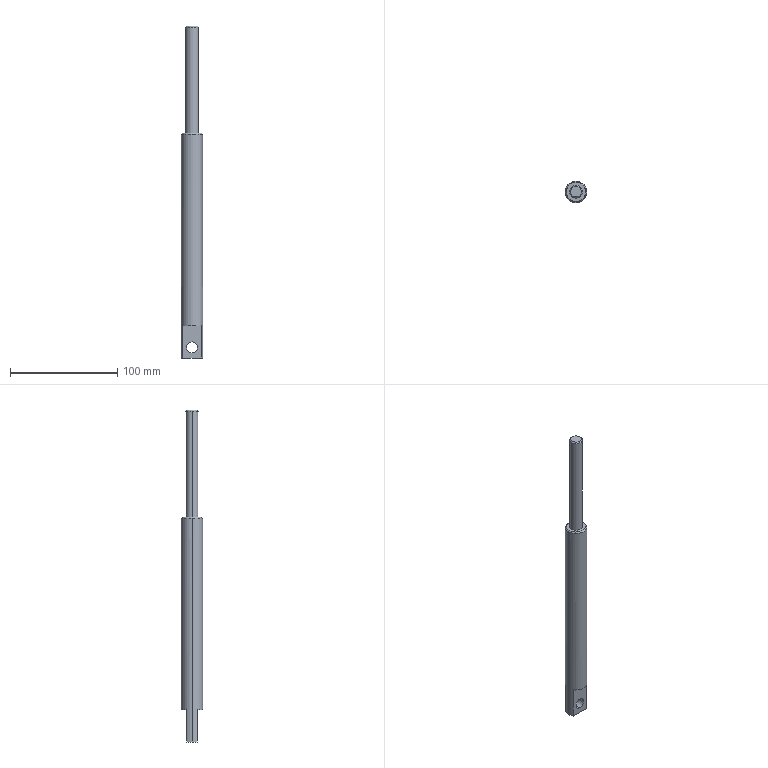Part | SolidWorks | features ICE 3, Chamfer 1, Extrusion 1 | 1 solid | 17 faces | box 20 x 20 x 310 mm | volume 72765 mm3 | plane 7 | cylinder 6 | cone 4 | commonest cylinder face diameters 10 x2 12 x2 20 x2
STEP:
#1=CARTESIAN_POINT('',(9.,0.,210.));
#2=VERTEX_POINT('',#1);
#3=CARTESIAN_POINT('',(-9.,0.,210.));
#4=VERTEX_POINT('',#3);
#5=CARTESIAN_POINT('',(0.,0.,210.));
#6=DIRECTION('',(0.,0.,1.));
#7=DIRECTION('',(1.,0.,0.));
#8=AXIS2_PLACEMENT_3D('',#5,#6,#7);
#9=CIRCLE('',#8,9.);
#10=EDGE_CURVE('',#2,#4,#9,.T.);
#11=ORIENTED_EDGE('',*,*,#10,.F.);
#12=CARTESIAN_POINT('',(10.,0.,209.));
#13=VERTEX_POINT('',#12);
#14=CARTESIAN_POINT('',(9.,0.,210.));
#15=DIRECTION('',(0.7071,0.,-0.7071));
#16=VECTOR('',#15,1000.);
#17=LINE('',#14,#16);
#18=EDGE_CURVE('',#2,#13,#17,.T.);
#19=ORIENTED_EDGE('',*,*,#18,.T.);
#20=CARTESIAN_POINT('',(-10.,0.,209.));
#21=VERTEX_POINT('',#20);
#22=CARTESIAN_POINT('',(0.,0.,209.));
#23=DIRECTION('',(0.,0.,-1.));
#24=DIRECTION('',(1.,0.,0.));
#25=AXIS2_PLACEMENT_3D('',#22,#23,#24);
#26=CIRCLE('',#25,10.);
#27=EDGE_CURVE('',#21,#13,#26,.T.);
#28=ORIENTED_EDGE('',*,*,#27,.F.);
#29=CARTESIAN_POINT('',(-9.,0.,210.));
#30=DIRECTION('',(-0.7071,0.,-0.7071));
#31=VECTOR('',#30,1000.);
#32=LINE('',#29,#31);
#33=EDGE_CURVE('',#4,#21,#32,.T.);
#34=ORIENTED_EDGE('',*,*,#33,.F.);
#35=EDGE_LOOP('',(#11,#19,#28,#34));
#36=FACE_OUTER_BOUND('',#35,.T.);
#37=CARTESIAN_POINT('',(0.,0.,210.));
#38=DIRECTION('',(0.,0.,-1.));
#39=DIRECTION('',(-1.,0.,0.));
#40=AXIS2_PLACEMENT_3D('',#37,#38,#39);
#41=CONICAL_SURFACE('',#40,9.,0.7854);
#42=ADVANCED_FACE('',(#36),#41,.T.);
#43=CARTESIAN_POINT('',(5.,0.,310.));
#44=VERTEX_POINT('',#43);
#45=CARTESIAN_POINT('',(-5.,0.,310.));
#46=VERTEX_POINT('',#45);
#47=CARTESIAN_POINT('',(0.,0.,310.));
#48=DIRECTION('',(0.,0.,1.));
#49=DIRECTION('',(1.,0.,0.));
#50=AXIS2_PLACEMENT_3D('',#47,#48,#49);
#51=CIRCLE('',#50,5.);
#52=EDGE_CURVE('',#44,#46,#51,.T.);
#53=ORIENTED_EDGE('',*,*,#52,.F.);
#54=CARTESIAN_POINT('',(6.,0.,309.));
#55=VERTEX_POINT('',#54);
#56=CARTESIAN_POINT('',(5.,0.,310.));
#57=DIRECTION('',(0.7071,0.,-0.7071));
#58=VECTOR('',#57,1000.);
#59=LINE('',#56,#58);
#60=EDGE_CURVE('',#44,#55,#59,.T.);
#61=ORIENTED_EDGE('',*,*,#60,.T.);
#62=CARTESIAN_POINT('',(-6.,0.,309.));
#63=VERTEX_POINT('',#62);
#64=CARTESIAN_POINT('',(0.,0.,309.));
#65=DIRECTION('',(0.,0.,-1.));
#66=DIRECTION('',(1.,0.,0.));
#67=AXIS2_PLACEMENT_3D('',#64,#65,#66);
#68=CIRCLE('',#67,6.);
#69=EDGE_CURVE('',#63,#55,#68,.T.);
#70=ORIENTED_EDGE('',*,*,#69,.F.);
#71=CARTESIAN_POINT('',(-5.,0.,310.));
#72=DIRECTION('',(-0.7071,0.,-0.7071));
#73=VECTOR('',#72,1000.);
#74=LINE('',#71,#73);
#75=EDGE_CURVE('',#46,#63,#74,.T.);
#76=ORIENTED_EDGE('',*,*,#75,.F.);
#77=EDGE_LOOP('',(#53,#61,#70,#76));
#78=FACE_OUTER_BOUND('',#77,.T.);
#79=CARTESIAN_POINT('',(0.,0.,310.));
#80=DIRECTION('',(0.,0.,-1.));
#81=DIRECTION('',(-1.,0.,0.));
#82=AXIS2_PLACEMENT_3D('',#79,#80,#81);
#83=CONICAL_SURFACE('',#82,5.,0.7854);
#84=ADVANCED_FACE('',(#78),#83,.T.);
#85=ORIENTED_EDGE('',*,*,#69,.T.);
#86=CARTESIAN_POINT('',(6.,0.,210.));
#87=VERTEX_POINT('',#86);
#88=CARTESIAN_POINT('',(6.,0.,310.));
#89=DIRECTION('',(0.,0.,-1.));
#90=VECTOR('',#89,1000.);
#91=LINE('',#88,#90);
#92=EDGE_CURVE('',#55,#87,#91,.T.);
#93=ORIENTED_EDGE('',*,*,#92,.T.);
#94=CARTESIAN_POINT('',(-6.,0.,210.));
#95=VERTEX_POINT('',#94);
#96=CARTESIAN_POINT('',(0.,0.,210.));
#97=DIRECTION('',(0.,0.,1.));
#98=DIRECTION('',(1.,0.,0.));
#99=AXIS2_PLACEMENT_3D('',#96,#97,#98);
#100=CIRCLE('',#99,6.);
#101=EDGE_CURVE('',#87,#95,#100,.T.);
#102=ORIENTED_EDGE('',*,*,#101,.T.);
#103=CARTESIAN_POINT('',(-6.,0.,310.));
#104=DIRECTION('',(0.,0.,-1.));
#105=VECTOR('',#104,1000.);
#106=LINE('',#103,#105);
#107=EDGE_CURVE('',#63,#95,#106,.T.);
#108=ORIENTED_EDGE('',*,*,#107,.F.);
#109=EDGE_LOOP('',(#85,#93,#102,#108));
#110=FACE_OUTER_BOUND('',#109,.T.);
#111=CARTESIAN_POINT('',(0.,0.,310.));
#112=DIRECTION('',(0.,0.,-1.));
#113=DIRECTION('',(-1.,0.,0.));
#114=AXIS2_PLACEMENT_3D('',#111,#112,#113);
#115=CYLINDRICAL_SURFACE('',#114,6.);
#116=ADVANCED_FACE('',(#110),#115,.T.);
#117=CARTESIAN_POINT('',(0.,-5.,5.));
#118=VERTEX_POINT('',#117);
#119=CARTESIAN_POINT('',(0.,-5.,15.));
#120=VERTEX_POINT('',#119);
#121=CARTESIAN_POINT('',(0.,-5.,10.));
#122=DIRECTION('',(0.,1.,0.));
#123=DIRECTION('',(0.,0.,-1.));
#124=AXIS2_PLACEMENT_3D('',#121,#122,#123);
#125=CIRCLE('',#124,5.);
#126=EDGE_CURVE('',#118,#120,#125,.T.);
#127=ORIENTED_EDGE('',*,*,#126,.F.);
#128=CARTESIAN_POINT('',(0.,5.,5.));
#129=VERTEX_POINT('',#128);
#130=CARTESIAN_POINT('',(0.,-10.,5.));
#131=DIRECTION('',(0.,1.,0.));
#132=VECTOR('',#131,1000.);
#133=LINE('',#130,#132);
#134=EDGE_CURVE('',#118,#129,#133,.T.);
#135=ORIENTED_EDGE('',*,*,#134,.T.);
#136=CARTESIAN_POINT('',(0.,5.,15.));
#137=VERTEX_POINT('',#136);
#138=CARTESIAN_POINT('',(0.,5.,10.));
#139=DIRECTION('',(0.,-1.,0.));
#140=DIRECTION('',(0.,0.,1.));
#141=AXIS2_PLACEMENT_3D('',#138,#139,#140);
#142=CIRCLE('',#141,5.);
#143=EDGE_CURVE('',#137,#129,#142,.T.);
#144=ORIENTED_EDGE('',*,*,#143,.F.);
#145=CARTESIAN_POINT('',(0.,-10.,15.));
#146=DIRECTION('',(0.,1.,0.));
#147=VECTOR('',#146,1000.);
#148=LINE('',#145,#147);
#149=EDGE_CURVE('',#120,#137,#148,.T.);
#150=ORIENTED_EDGE('',*,*,#149,.F.);
#151=EDGE_LOOP('',(#127,#135,#144,#150));
#152=FACE_OUTER_BOUND('',#151,.T.);
#153=CARTESIAN_POINT('',(0.,-10.,10.));
#154=DIRECTION('',(0.,1.,0.));
#155=DIRECTION('',(0.,0.,1.));
#156=AXIS2_PLACEMENT_3D('',#153,#154,#155);
#157=CYLINDRICAL_SURFACE('',#156,5.);
#158=ADVANCED_FACE('',(#152),#157,.F.);
#159=ORIENTED_EDGE('',*,*,#27,.T.);
#160=CARTESIAN_POINT('',(10.,0.,0.));
#161=VERTEX_POINT('',#160);
#162=CARTESIAN_POINT('',(10.,0.,210.));
#163=DIRECTION('',(0.,0.,-1.));
#164=VECTOR('',#163,1000.);
#165=LINE('',#162,#164);
#166=EDGE_CURVE('',#13,#161,#165,.T.);
#167=ORIENTED_EDGE('',*,*,#166,.T.);
#168=CARTESIAN_POINT('',(8.66,5.,0.));
#169=VERTEX_POINT('',#168);
#170=CARTESIAN_POINT('',(0.,0.,0.));
#171=DIRECTION('',(0.,0.,1.));
#172=DIRECTION('',(1.,0.,0.));
#173=AXIS2_PLACEMENT_3D('',#170,#171,#172);
#174=CIRCLE('',#173,10.);
#175=EDGE_CURVE('',#161,#169,#174,.T.);
#176=ORIENTED_EDGE('',*,*,#175,.T.);
#177=CARTESIAN_POINT('',(8.66,5.,30.));
#178=VERTEX_POINT('',#177);
#179=CARTESIAN_POINT('',(8.66,5.,210.));
#180=DIRECTION('',(0.,0.,-1.));
#181=VECTOR('',#180,1000.);
#182=LINE('',#179,#181);
#183=EDGE_CURVE('',#178,#169,#182,.T.);
#184=ORIENTED_EDGE('',*,*,#183,.F.);
#185=CARTESIAN_POINT('',(-8.66,5.,30.));
#186=VERTEX_POINT('',#185);
#187=CARTESIAN_POINT('',(0.,0.,30.));
#188=DIRECTION('',(0.,0.,-1.));
#189=DIRECTION('',(-1.,0.,0.));
#190=AXIS2_PLACEMENT_3D('',#187,#188,#189);
#191=CIRCLE('',#190,10.);
#192=EDGE_CURVE('',#186,#178,#191,.T.);
#193=ORIENTED_EDGE('',*,*,#192,.F.);
#194=CARTESIAN_POINT('',(-8.66,5.,0.));
#195=VERTEX_POINT('',#194);
#196=CARTESIAN_POINT('',(-8.66,5.,210.));
#197=DIRECTION('',(0.,0.,1.));
#198=VECTOR('',#197,1000.);
#199=LINE('',#196,#198);
#200=EDGE_CURVE('',#195,#186,#199,.T.);
#201=ORIENTED_EDGE('',*,*,#200,.F.);
#202=CARTESIAN_POINT('',(-10.,0.,0.));
#203=VERTEX_POINT('',#202);
#204=CARTESIAN_POINT('',(0.,0.,0.));
#205=DIRECTION('',(0.,0.,1.));
#206=DIRECTION('',(1.,0.,0.));
#207=AXIS2_PLACEMENT_3D('',#204,#205,#206);
#208=CIRCLE('',#207,10.);
#209=EDGE_CURVE('',#195,#203,#208,.T.);
#210=ORIENTED_EDGE('',*,*,#209,.T.);
#211=CARTESIAN_POINT('',(-10.,0.,210.));
#212=DIRECTION('',(0.,0.,-1.));
#213=VECTOR('',#212,1000.);
#214=LINE('',#211,#213);
#215=EDGE_CURVE('',#21,#203,#214,.T.);
#216=ORIENTED_EDGE('',*,*,#215,.F.);
#217=EDGE_LOOP('',(#159,#167,#176,#184,#193,#201,#210,#216));
#218=FACE_OUTER_BOUND('',#217,.T.);
#219=CARTESIAN_POINT('',(0.,0.,210.));
#220=DIRECTION('',(0.,0.,-1.));
#221=DIRECTION('',(-1.,0.,0.));
#222=AXIS2_PLACEMENT_3D('',#219,#220,#221);
#223=CYLINDRICAL_SURFACE('',#222,10.);
#224=ADVANCED_FACE('',(#218),#223,.T.);
#225=ORIENTED_EDGE('',*,*,#166,.F.);
#226=CARTESIAN_POINT('',(0.,0.,209.));
#227=DIRECTION('',(0.,0.,-1.));
#228=DIRECTION('',(1.,0.,0.));
#229=AXIS2_PLACEMENT_3D('',#226,#227,#228);
#230=CIRCLE('',#229,10.);
#231=EDGE_CURVE('',#13,#21,#230,.T.);
#232=ORIENTED_EDGE('',*,*,#231,.T.);
#233=ORIENTED_EDGE('',*,*,#215,.T.);
#234=CARTESIAN_POINT('',(-8.66,-5.,0.));
#235=VERTEX_POINT('',#234);
#236=CARTESIAN_POINT('',(0.,0.,0.));
#237=DIRECTION('',(0.,0.,1.));
#238=DIRECTION('',(1.,0.,0.));
#239=AXIS2_PLACEMENT_3D('',#236,#237,#238);
#240=CIRCLE('',#239,10.);
#241=EDGE_CURVE('',#203,#235,#240,.T.);
#242=ORIENTED_EDGE('',*,*,#241,.T.);
#243=CARTESIAN_POINT('',(-8.66,-5.,30.));
#244=VERTEX_POINT('',#243);
#245=CARTESIAN_POINT('',(-8.66,-5.,210.));
#246=DIRECTION('',(0.,0.,-1.));
#247=VECTOR('',#246,1000.);
#248=LINE('',#245,#247);
#249=EDGE_CURVE('',#244,#235,#248,.T.);
#250=ORIENTED_EDGE('',*,*,#249,.F.);
#251=CARTESIAN_POINT('',(8.66,-5.,30.));
#252=VERTEX_POINT('',#251);
#253=CARTESIAN_POINT('',(0.,0.,30.));
#254=DIRECTION('',(0.,0.,-1.));
#255=DIRECTION('',(-1.,0.,0.));
#256=AXIS2_PLACEMENT_3D('',#253,#254,#255);
#257=CIRCLE('',#256,10.);
#258=EDGE_CURVE('',#252,#244,#257,.T.);
#259=ORIENTED_EDGE('',*,*,#258,.F.);
#260=CARTESIAN_POINT('',(8.66,-5.,0.));
#261=VERTEX_POINT('',#260);
#262=CARTESIAN_POINT('',(8.66,-5.,210.));
#263=DIRECTION('',(0.,0.,1.));
#264=VECTOR('',#263,1000.);
#265=LINE('',#262,#264);
#266=EDGE_CURVE('',#261,#252,#265,.T.);
#267=ORIENTED_EDGE('',*,*,#266,.F.);
#268=CARTESIAN_POINT('',(0.,0.,0.));
#269=DIRECTION('',(0.,0.,1.));
#270=DIRECTION('',(1.,0.,0.));
#271=AXIS2_PLACEMENT_3D('',#268,#269,#270);
#272=CIRCLE('',#271,10.);
#273=EDGE_CURVE('',#261,#161,#272,.T.);
#274=ORIENTED_EDGE('',*,*,#273,.T.);
#275=EDGE_LOOP('',(#225,#232,#233,#242,#250,#259,#267,#274));
#276=FACE_OUTER_BOUND('',#275,.T.);
#277=CARTESIAN_POINT('',(0.,0.,210.));
#278=DIRECTION('',(0.,0.,-1.));
#279=DIRECTION('',(-1.,0.,0.));
#280=AXIS2_PLACEMENT_3D('',#277,#278,#279);
#281=CYLINDRICAL_SURFACE('',#280,10.);
#282=ADVANCED_FACE('',(#276),#281,.T.);
#283=CARTESIAN_POINT('',(0.,-5.,0.));
#284=DIRECTION('',(1.,0.,0.));
#285=VECTOR('',#284,1000.);
#286=LINE('',#283,#285);
#287=EDGE_CURVE('',#235,#261,#286,.T.);
#288=ORIENTED_EDGE('',*,*,#287,.F.);
#289=ORIENTED_EDGE('',*,*,#241,.F.);
#290=ORIENTED_EDGE('',*,*,#209,.F.);
#291=CARTESIAN_POINT('',(0.,5.,0.));
#292=DIRECTION('',(-1.,0.,0.));
#293=VECTOR('',#292,1000.);
#294=LINE('',#291,#293);
#295=EDGE_CURVE('',#169,#195,#294,.T.);
#296=ORIENTED_EDGE('',*,*,#295,.F.);
#297=ORIENTED_EDGE('',*,*,#175,.F.);
#298=ORIENTED_EDGE('',*,*,#273,.F.);
#299=EDGE_LOOP('',(#288,#289,#290,#296,#297,#298));
#300=FACE_OUTER_BOUND('',#299,.T.);
#301=CARTESIAN_POINT('',(0.,0.,0.));
#302=DIRECTION('',(0.,0.,1.));
#303=DIRECTION('',(1.,0.,0.));
#304=AXIS2_PLACEMENT_3D('',#301,#302,#303);
#305=PLANE('',#304);
#306=ADVANCED_FACE('',(#300),#305,.F.);
#307=CARTESIAN_POINT('',(0.,0.,210.));
#308=DIRECTION('',(0.,0.,1.));
#309=DIRECTION('',(1.,0.,0.));
#310=AXIS2_PLACEMENT_3D('',#307,#308,#309);
#311=CIRCLE('',#310,9.);
#312=EDGE_CURVE('',#4,#2,#311,.T.);
#313=ORIENTED_EDGE('',*,*,#312,.T.);
#314=ORIENTED_EDGE('',*,*,#10,.T.);
#315=EDGE_LOOP('',(#313,#314));
#316=FACE_OUTER_BOUND('',#315,.T.);
#317=CARTESIAN_POINT('',(0.,0.,210.));
#318=DIRECTION('',(0.,0.,1.));
#319=DIRECTION('',(1.,0.,0.));
#320=AXIS2_PLACEMENT_3D('',#317,#318,#319);
#321=CIRCLE('',#320,6.);
#322=EDGE_CURVE('',#95,#87,#321,.T.);
#323=ORIENTED_EDGE('',*,*,#322,.F.);
#324=ORIENTED_EDGE('',*,*,#101,.F.);
#325=EDGE_LOOP('',(#323,#324));
#326=FACE_BOUND('',#325,.T.);
#327=CARTESIAN_POINT('',(0.,0.,210.));
#328=DIRECTION('',(0.,0.,1.));
#329=DIRECTION('',(1.,0.,0.));
#330=AXIS2_PLACEMENT_3D('',#327,#328,#329);
#331=PLANE('',#330);
#332=ADVANCED_FACE('',(#316,#326),#331,.T.);
#333=ORIENTED_EDGE('',*,*,#192,.T.);
#334=CARTESIAN_POINT('',(15.267,5.,30.));
#335=DIRECTION('',(-1.,0.,0.));
#336=VECTOR('',#335,1000.);
#337=LINE('',#334,#336);
#338=EDGE_CURVE('',#178,#186,#337,.T.);
#339=ORIENTED_EDGE('',*,*,#338,.T.);
#340=EDGE_LOOP('',(#333,#339));
#341=FACE_OUTER_BOUND('',#340,.T.);
#342=CARTESIAN_POINT('',(0.,0.,30.));
#343=DIRECTION('',(0.,0.,-1.));
#344=DIRECTION('',(-1.,0.,0.));
#345=AXIS2_PLACEMENT_3D('',#342,#343,#344);
#346=PLANE('',#345);
#347=ADVANCED_FACE('',(#341),#346,.T.);
#348=ORIENTED_EDGE('',*,*,#143,.T.);
#349=CARTESIAN_POINT('',(0.,5.,10.));
#350=DIRECTION('',(0.,-1.,0.));
#351=DIRECTION('',(0.,0.,1.));
#352=AXIS2_PLACEMENT_3D('',#349,#350,#351);
#353=CIRCLE('',#352,5.);
#354=EDGE_CURVE('',#129,#137,#353,.T.);
#355=ORIENTED_EDGE('',*,*,#354,.T.);
#356=EDGE_LOOP('',(#348,#355));
#357=FACE_BOUND('',#356,.T.);
#358=ORIENTED_EDGE('',*,*,#183,.T.);
#359=ORIENTED_EDGE('',*,*,#295,.T.);
#360=ORIENTED_EDGE('',*,*,#200,.T.);
#361=ORIENTED_EDGE('',*,*,#338,.F.);
#362=EDGE_LOOP('',(#358,#359,#360,#361));
#363=FACE_OUTER_BOUND('',#362,.T.);
#364=CARTESIAN_POINT('',(15.267,5.,-0.000012));
#365=DIRECTION('',(0.,1.,0.));
#366=DIRECTION('',(0.,0.,1.));
#367=AXIS2_PLACEMENT_3D('',#364,#365,#366);
#368=PLANE('',#367);
#369=ADVANCED_FACE('',(#357,#363),#368,.T.);
#370=ORIENTED_EDGE('',*,*,#258,.T.);
#371=CARTESIAN_POINT('',(18.488,-5.,30.));
#372=DIRECTION('',(1.,0.,0.));
#373=VECTOR('',#372,1000.);
#374=LINE('',#371,#373);
#375=EDGE_CURVE('',#244,#252,#374,.T.);
#376=ORIENTED_EDGE('',*,*,#375,.T.);
#377=EDGE_LOOP('',(#370,#376));
#378=FACE_OUTER_BOUND('',#377,.T.);
#379=CARTESIAN_POINT('',(0.,0.,30.));
#380=DIRECTION('',(0.,0.,-1.));
#381=DIRECTION('',(-1.,0.,0.));
#382=AXIS2_PLACEMENT_3D('',#379,#380,#381);
#383=PLANE('',#382);
#384=ADVANCED_FACE('',(#378),#383,.T.);
#385=CARTESIAN_POINT('',(0.,-5.,10.));
#386=DIRECTION('',(0.,1.,0.));
#387=DIRECTION('',(0.,0.,-1.));
#388=AXIS2_PLACEMENT_3D('',#385,#386,#387);
#389=CIRCLE('',#388,5.);
#390=EDGE_CURVE('',#120,#118,#389,.T.);
#391=ORIENTED_EDGE('',*,*,#390,.T.);
#392=ORIENTED_EDGE('',*,*,#126,.T.);
#393=EDGE_LOOP('',(#391,#392));
#394=FACE_BOUND('',#393,.T.);
#395=ORIENTED_EDGE('',*,*,#249,.T.);
#396=ORIENTED_EDGE('',*,*,#287,.T.);
#397=ORIENTED_EDGE('',*,*,#266,.T.);
#398=ORIENTED_EDGE('',*,*,#375,.F.);
#399=EDGE_LOOP('',(#395,#396,#397,#398));
#400=FACE_OUTER_BOUND('',#399,.T.);
#401=CARTESIAN_POINT('',(18.488,-5.,-0.000012));
#402=DIRECTION('',(0.,-1.,0.));
#403=DIRECTION('',(0.,0.,-1.));
#404=AXIS2_PLACEMENT_3D('',#401,#402,#403);
#405=PLANE('',#404);
#406=ADVANCED_FACE('',(#394,#400),#405,.T.);
#407=ORIENTED_EDGE('',*,*,#134,.F.);
#408=ORIENTED_EDGE('',*,*,#390,.F.);
#409=ORIENTED_EDGE('',*,*,#149,.T.);
#410=ORIENTED_EDGE('',*,*,#354,.F.);
#411=EDGE_LOOP('',(#407,#408,#409,#410));
#412=FACE_OUTER_BOUND('',#411,.T.);
#413=CARTESIAN_POINT('',(0.,-10.,10.));
#414=DIRECTION('',(0.,1.,0.));
#415=DIRECTION('',(0.,0.,1.));
#416=AXIS2_PLACEMENT_3D('',#413,#414,#415);
#417=CYLINDRICAL_SURFACE('',#416,5.);
#418=ADVANCED_FACE('',(#412),#417,.F.);
#419=ORIENTED_EDGE('',*,*,#92,.F.);
#420=CARTESIAN_POINT('',(0.,0.,309.));
#421=DIRECTION('',(0.,0.,-1.));
#422=DIRECTION('',(1.,0.,0.));
#423=AXIS2_PLACEMENT_3D('',#420,#421,#422);
#424=CIRCLE('',#423,6.);
#425=EDGE_CURVE('',#55,#63,#424,.T.);
#426=ORIENTED_EDGE('',*,*,#425,.T.);
#427=ORIENTED_EDGE('',*,*,#107,.T.);
#428=ORIENTED_EDGE('',*,*,#322,.T.);
#429=EDGE_LOOP('',(#419,#426,#427,#428));
#430=FACE_OUTER_BOUND('',#429,.T.);
#431=CARTESIAN_POINT('',(0.,0.,310.));
#432=DIRECTION('',(0.,0.,-1.));
#433=DIRECTION('',(-1.,0.,0.));
#434=AXIS2_PLACEMENT_3D('',#431,#432,#433);
#435=CYLINDRICAL_SURFACE('',#434,6.);
#436=ADVANCED_FACE('',(#430),#435,.T.);
#437=CARTESIAN_POINT('',(0.,0.,310.));
#438=DIRECTION('',(0.,0.,1.));
#439=DIRECTION('',(1.,0.,0.));
#440=AXIS2_PLACEMENT_3D('',#437,#438,#439);
#441=CIRCLE('',#440,5.);
#442=EDGE_CURVE('',#46,#44,#441,.T.);
#443=ORIENTED_EDGE('',*,*,#442,.T.);
#444=ORIENTED_EDGE('',*,*,#52,.T.);
#445=EDGE_LOOP('',(#443,#444));
#446=FACE_OUTER_BOUND('',#445,.T.);
#447=CARTESIAN_POINT('',(0.,0.,310.));
#448=DIRECTION('',(0.,0.,1.));
#449=DIRECTION('',(1.,0.,0.));
#450=AXIS2_PLACEMENT_3D('',#447,#448,#449);
#451=PLANE('',#450);
#452=ADVANCED_FACE('',(#446),#451,.T.);
#453=ORIENTED_EDGE('',*,*,#60,.F.);
#454=ORIENTED_EDGE('',*,*,#442,.F.);
#455=ORIENTED_EDGE('',*,*,#75,.T.);
#456=ORIENTED_EDGE('',*,*,#425,.F.);
#457=EDGE_LOOP('',(#453,#454,#455,#456));
#458=FACE_OUTER_BOUND('',#457,.T.);
#459=CARTESIAN_POINT('',(0.,0.,310.));
#460=DIRECTION('',(0.,0.,-1.));
#461=DIRECTION('',(-1.,0.,0.));
#462=AXIS2_PLACEMENT_3D('',#459,#460,#461);
#463=CONICAL_SURFACE('',#462,5.,0.7854);
#464=ADVANCED_FACE('',(#458),#463,.T.);
#465=ORIENTED_EDGE('',*,*,#18,.F.);
#466=ORIENTED_EDGE('',*,*,#312,.F.);
#467=ORIENTED_EDGE('',*,*,#33,.T.);
#468=ORIENTED_EDGE('',*,*,#231,.F.);
#469=EDGE_LOOP('',(#465,#466,#467,#468));
#470=FACE_OUTER_BOUND('',#469,.T.);
#471=CARTESIAN_POINT('',(0.,0.,210.));
#472=DIRECTION('',(0.,0.,-1.));
#473=DIRECTION('',(-1.,0.,0.));
#474=AXIS2_PLACEMENT_3D('',#471,#472,#473);
#475=CONICAL_SURFACE('',#474,9.,0.7854);
#476=ADVANCED_FACE('',(#470),#475,.T.);
#477=CLOSED_SHELL('',(#42,#84,#116,#158,#224,#282,#306,#332,#347,#369,#384,#406,#418,#436,#452,#464,#476));
#478=MANIFOLD_SOLID_BREP('',#477);
#479=CARTESIAN_POINT('',(0.,0.,0.));
#480=DIRECTION('',(0.,0.,1.));
#481=DIRECTION('',(1.,0.,0.));
#482=AXIS2_PLACEMENT_3D('',#479,#480,#481);
#483=(LENGTH_UNIT()NAMED_UNIT(*)SI_UNIT(.MILLI.,.METRE.));
#484=UNCERTAINTY_MEASURE_WITH_UNIT(LENGTH_MEASURE(0.00001),#483,'','');
#485=(NAMED_UNIT(*)PLANE_ANGLE_UNIT()SI_UNIT($,.RADIAN.));
#486=(NAMED_UNIT(*)SI_UNIT($,.STERADIAN.)SOLID_ANGLE_UNIT());
#487=(GEOMETRIC_REPRESENTATION_CONTEXT(3)GLOBAL_UNCERTAINTY_ASSIGNED_CONTEXT((#484))GLOBAL_UNIT_ASSIGNED_CONTEXT((#483,#485,#486))REPRESENTATION_CONTEXT('',''));
#488=ADVANCED_BREP_SHAPE_REPRESENTATION('',(#478,#482),#487);